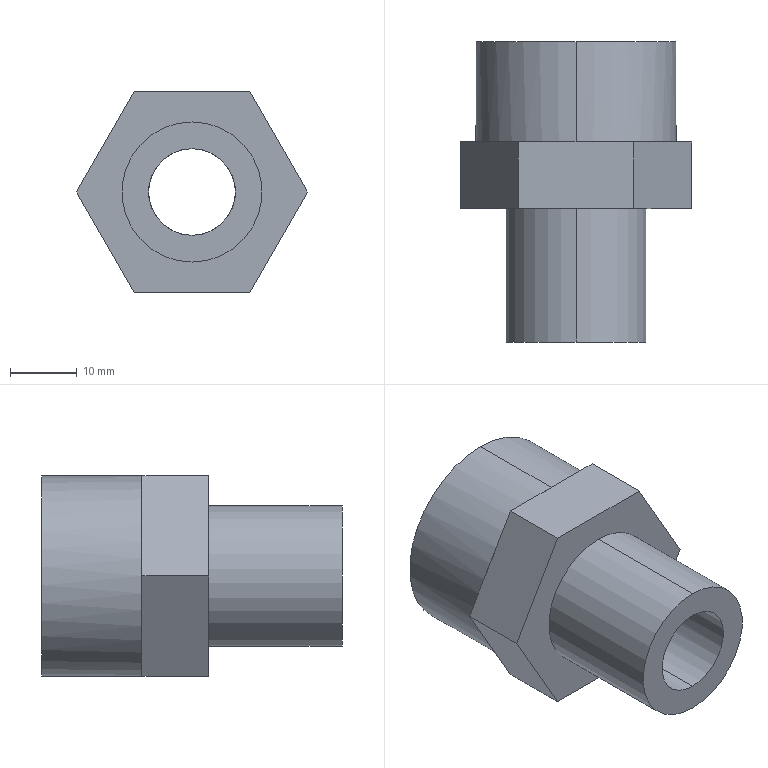Part | 1 solid | 23 faces | box 34.641 x 45 x 30 mm | volume 18087 mm3 | plane 15 | cylinder 6 | cone 2 | commonest cylinder face diameters 13 x2 21 x2 30 x2
STEP:
#1=CARTESIAN_POINT('',(6.5,30.,0.));
#2=VERTEX_POINT('',#1);
#3=CARTESIAN_POINT('',(0.,30.,-6.5));
#4=VERTEX_POINT('',#3);
#5=CARTESIAN_POINT('',(0.,30.,0.));
#6=DIRECTION('',(0.,1.,0.));
#7=DIRECTION('',(-1.,0.,0.));
#8=AXIS2_PLACEMENT_3D('',#5,#6,#7);
#9=CIRCLE('',#8,6.5);
#10=EDGE_CURVE('',#2,#4,#9,.T.);
#11=ORIENTED_EDGE('',*,*,#10,.F.);
#12=CARTESIAN_POINT('',(10.,45.,0.));
#13=VERTEX_POINT('',#12);
#14=CARTESIAN_POINT('',(10.,45.,0.));
#15=DIRECTION('',(0.2272,0.9738,0.));
#16=VECTOR('',#15,1000.);
#17=LINE('',#14,#16);
#18=EDGE_CURVE('',#2,#13,#17,.T.);
#19=ORIENTED_EDGE('',*,*,#18,.T.);
#20=CARTESIAN_POINT('',(-10.,45.,0.));
#21=VERTEX_POINT('',#20);
#22=CARTESIAN_POINT('',(0.,45.,0.));
#23=DIRECTION('',(0.,1.,0.));
#24=DIRECTION('',(-1.,0.,0.));
#25=AXIS2_PLACEMENT_3D('',#22,#23,#24);
#26=CIRCLE('',#25,10.);
#27=EDGE_CURVE('',#13,#21,#26,.T.);
#28=ORIENTED_EDGE('',*,*,#27,.T.);
#29=CARTESIAN_POINT('',(-6.5,30.,0.));
#30=VERTEX_POINT('',#29);
#31=CARTESIAN_POINT('',(-10.,45.,0.));
#32=DIRECTION('',(-0.2272,0.9738,0.));
#33=VECTOR('',#32,1000.);
#34=LINE('',#31,#33);
#35=EDGE_CURVE('',#30,#21,#34,.T.);
#36=ORIENTED_EDGE('',*,*,#35,.F.);
#37=CARTESIAN_POINT('',(0.,30.,0.));
#38=DIRECTION('',(0.,1.,0.));
#39=DIRECTION('',(-1.,0.,0.));
#40=AXIS2_PLACEMENT_3D('',#37,#38,#39);
#41=CIRCLE('',#40,6.5);
#42=EDGE_CURVE('',#4,#30,#41,.T.);
#43=ORIENTED_EDGE('',*,*,#42,.F.);
#44=EDGE_LOOP('',(#11,#19,#28,#36,#43));
#45=FACE_OUTER_BOUND('',#44,.T.);
#46=CARTESIAN_POINT('',(0.,45.,0.));
#47=DIRECTION('',(0.,1.,0.));
#48=DIRECTION('',(-1.,0.,0.));
#49=AXIS2_PLACEMENT_3D('',#46,#47,#48);
#50=CONICAL_SURFACE('',#49,10.,0.2292);
#51=ADVANCED_FACE('',(#45),#50,.F.);
#52=CARTESIAN_POINT('',(0.,0.,-6.5));
#53=VERTEX_POINT('',#52);
#54=CARTESIAN_POINT('',(0.,0.,6.5));
#55=VERTEX_POINT('',#54);
#56=CARTESIAN_POINT('',(0.,0.,0.));
#57=DIRECTION('',(0.,1.,0.));
#58=DIRECTION('',(0.,0.,1.));
#59=AXIS2_PLACEMENT_3D('',#56,#57,#58);
#60=CIRCLE('',#59,6.5);
#61=EDGE_CURVE('',#53,#55,#60,.T.);
#62=ORIENTED_EDGE('',*,*,#61,.F.);
#63=CARTESIAN_POINT('',(0.,0.,-6.5));
#64=DIRECTION('',(0.,1.,0.));
#65=VECTOR('',#64,1000.);
#66=LINE('',#63,#65);
#67=EDGE_CURVE('',#53,#4,#66,.T.);
#68=ORIENTED_EDGE('',*,*,#67,.T.);
#69=ORIENTED_EDGE('',*,*,#42,.T.);
#70=CARTESIAN_POINT('',(0.,30.,6.5));
#71=VERTEX_POINT('',#70);
#72=CARTESIAN_POINT('',(0.,30.,0.));
#73=DIRECTION('',(0.,1.,0.));
#74=DIRECTION('',(-1.,0.,0.));
#75=AXIS2_PLACEMENT_3D('',#72,#73,#74);
#76=CIRCLE('',#75,6.5);
#77=EDGE_CURVE('',#30,#71,#76,.T.);
#78=ORIENTED_EDGE('',*,*,#77,.T.);
#79=CARTESIAN_POINT('',(0.,0.,6.5));
#80=DIRECTION('',(0.,1.,0.));
#81=VECTOR('',#80,1000.);
#82=LINE('',#79,#81);
#83=EDGE_CURVE('',#55,#71,#82,.T.);
#84=ORIENTED_EDGE('',*,*,#83,.F.);
#85=EDGE_LOOP('',(#62,#68,#69,#78,#84));
#86=FACE_OUTER_BOUND('',#85,.T.);
#87=CARTESIAN_POINT('',(0.,0.,0.));
#88=DIRECTION('',(0.,1.,0.));
#89=DIRECTION('',(0.,0.,1.));
#90=AXIS2_PLACEMENT_3D('',#87,#88,#89);
#91=CYLINDRICAL_SURFACE('',#90,6.5);
#92=ADVANCED_FACE('',(#86),#91,.F.);
#93=CARTESIAN_POINT('',(0.,45.,15.));
#94=VERTEX_POINT('',#93);
#95=CARTESIAN_POINT('',(0.,45.,-15.));
#96=VERTEX_POINT('',#95);
#97=CARTESIAN_POINT('',(0.,45.,0.));
#98=DIRECTION('',(0.,1.,0.));
#99=DIRECTION('',(0.,0.,1.));
#100=AXIS2_PLACEMENT_3D('',#97,#98,#99);
#101=CIRCLE('',#100,15.);
#102=EDGE_CURVE('',#94,#96,#101,.T.);
#103=ORIENTED_EDGE('',*,*,#102,.F.);
#104=CARTESIAN_POINT('',(0.,30.,15.));
#105=VERTEX_POINT('',#104);
#106=CARTESIAN_POINT('',(0.,87.426,15.));
#107=DIRECTION('',(0.,-1.,0.));
#108=VECTOR('',#107,1000.);
#109=LINE('',#106,#108);
#110=EDGE_CURVE('',#94,#105,#109,.T.);
#111=ORIENTED_EDGE('',*,*,#110,.T.);
#112=CARTESIAN_POINT('',(12.99,30.,7.5));
#113=VERTEX_POINT('',#112);
#114=CARTESIAN_POINT('',(0.,30.,0.));
#115=DIRECTION('',(0.,1.,0.));
#116=DIRECTION('',(0.,0.,1.));
#117=AXIS2_PLACEMENT_3D('',#114,#115,#116);
#118=CIRCLE('',#117,15.);
#119=EDGE_CURVE('',#105,#113,#118,.T.);
#120=ORIENTED_EDGE('',*,*,#119,.T.);
#121=CARTESIAN_POINT('',(12.99,30.,-7.5));
#122=VERTEX_POINT('',#121);
#123=CARTESIAN_POINT('',(0.,30.,0.));
#124=DIRECTION('',(0.,1.,0.));
#125=DIRECTION('',(0.,0.,1.));
#126=AXIS2_PLACEMENT_3D('',#123,#124,#125);
#127=CIRCLE('',#126,15.);
#128=EDGE_CURVE('',#113,#122,#127,.T.);
#129=ORIENTED_EDGE('',*,*,#128,.T.);
#130=CARTESIAN_POINT('',(0.,30.,-15.));
#131=VERTEX_POINT('',#130);
#132=CARTESIAN_POINT('',(0.,30.,0.));
#133=DIRECTION('',(0.,1.,0.));
#134=DIRECTION('',(0.,0.,1.));
#135=AXIS2_PLACEMENT_3D('',#132,#133,#134);
#136=CIRCLE('',#135,15.);
#137=EDGE_CURVE('',#122,#131,#136,.T.);
#138=ORIENTED_EDGE('',*,*,#137,.T.);
#139=CARTESIAN_POINT('',(0.,87.426,-15.));
#140=DIRECTION('',(0.,-1.,0.));
#141=VECTOR('',#140,1000.);
#142=LINE('',#139,#141);
#143=EDGE_CURVE('',#96,#131,#142,.T.);
#144=ORIENTED_EDGE('',*,*,#143,.F.);
#145=EDGE_LOOP('',(#103,#111,#120,#129,#138,#144));
#146=FACE_OUTER_BOUND('',#145,.T.);
#147=CARTESIAN_POINT('',(0.,87.426,0.));
#148=DIRECTION('',(0.,-1.,0.));
#149=DIRECTION('',(0.,0.,-1.));
#150=AXIS2_PLACEMENT_3D('',#147,#148,#149);
#151=CYLINDRICAL_SURFACE('',#150,15.);
#152=ADVANCED_FACE('',(#146),#151,.T.);
#153=CARTESIAN_POINT('',(0.,20.,10.5));
#154=VERTEX_POINT('',#153);
#155=CARTESIAN_POINT('',(0.,20.,-10.5));
#156=VERTEX_POINT('',#155);
#157=CARTESIAN_POINT('',(0.,20.,0.));
#158=DIRECTION('',(0.,1.,0.));
#159=DIRECTION('',(0.,0.,1.));
#160=AXIS2_PLACEMENT_3D('',#157,#158,#159);
#161=CIRCLE('',#160,10.5);
#162=EDGE_CURVE('',#154,#156,#161,.T.);
#163=ORIENTED_EDGE('',*,*,#162,.F.);
#164=CARTESIAN_POINT('',(0.,0.,10.5));
#165=VERTEX_POINT('',#164);
#166=CARTESIAN_POINT('',(0.,45.,10.5));
#167=DIRECTION('',(0.,-1.,0.));
#168=VECTOR('',#167,1000.);
#169=LINE('',#166,#168);
#170=EDGE_CURVE('',#154,#165,#169,.T.);
#171=ORIENTED_EDGE('',*,*,#170,.T.);
#172=CARTESIAN_POINT('',(0.,0.,-10.5));
#173=VERTEX_POINT('',#172);
#174=CARTESIAN_POINT('',(0.,0.,0.));
#175=DIRECTION('',(0.,1.,0.));
#176=DIRECTION('',(0.,0.,1.));
#177=AXIS2_PLACEMENT_3D('',#174,#175,#176);
#178=CIRCLE('',#177,10.5);
#179=EDGE_CURVE('',#165,#173,#178,.T.);
#180=ORIENTED_EDGE('',*,*,#179,.T.);
#181=CARTESIAN_POINT('',(0.,45.,-10.5));
#182=DIRECTION('',(0.,-1.,0.));
#183=VECTOR('',#182,1000.);
#184=LINE('',#181,#183);
#185=EDGE_CURVE('',#156,#173,#184,.T.);
#186=ORIENTED_EDGE('',*,*,#185,.F.);
#187=EDGE_LOOP('',(#163,#171,#180,#186));
#188=FACE_OUTER_BOUND('',#187,.T.);
#189=CARTESIAN_POINT('',(0.,45.,0.));
#190=DIRECTION('',(0.,-1.,0.));
#191=DIRECTION('',(0.,0.,-1.));
#192=AXIS2_PLACEMENT_3D('',#189,#190,#191);
#193=CYLINDRICAL_SURFACE('',#192,10.5);
#194=ADVANCED_FACE('',(#188),#193,.T.);
#195=ORIENTED_EDGE('',*,*,#170,.F.);
#196=CARTESIAN_POINT('',(0.,20.,0.));
#197=DIRECTION('',(0.,1.,0.));
#198=DIRECTION('',(0.,0.,1.));
#199=AXIS2_PLACEMENT_3D('',#196,#197,#198);
#200=CIRCLE('',#199,10.5);
#201=EDGE_CURVE('',#156,#154,#200,.T.);
#202=ORIENTED_EDGE('',*,*,#201,.F.);
#203=ORIENTED_EDGE('',*,*,#185,.T.);
#204=CARTESIAN_POINT('',(0.,0.,0.));
#205=DIRECTION('',(0.,1.,0.));
#206=DIRECTION('',(0.,0.,1.));
#207=AXIS2_PLACEMENT_3D('',#204,#205,#206);
#208=CIRCLE('',#207,10.5);
#209=EDGE_CURVE('',#173,#165,#208,.T.);
#210=ORIENTED_EDGE('',*,*,#209,.T.);
#211=EDGE_LOOP('',(#195,#202,#203,#210));
#212=FACE_OUTER_BOUND('',#211,.T.);
#213=CARTESIAN_POINT('',(0.,45.,0.));
#214=DIRECTION('',(0.,-1.,0.));
#215=DIRECTION('',(0.,0.,-1.));
#216=AXIS2_PLACEMENT_3D('',#213,#214,#215);
#217=CYLINDRICAL_SURFACE('',#216,10.5);
#218=ADVANCED_FACE('',(#212),#217,.T.);
#219=CARTESIAN_POINT('',(0.,0.,0.));
#220=DIRECTION('',(0.,1.,0.));
#221=DIRECTION('',(0.,0.,1.));
#222=AXIS2_PLACEMENT_3D('',#219,#220,#221);
#223=CIRCLE('',#222,6.5);
#224=EDGE_CURVE('',#55,#53,#223,.T.);
#225=ORIENTED_EDGE('',*,*,#224,.T.);
#226=ORIENTED_EDGE('',*,*,#61,.T.);
#227=EDGE_LOOP('',(#225,#226));
#228=FACE_BOUND('',#227,.T.);
#229=ORIENTED_EDGE('',*,*,#209,.F.);
#230=ORIENTED_EDGE('',*,*,#179,.F.);
#231=EDGE_LOOP('',(#229,#230));
#232=FACE_OUTER_BOUND('',#231,.T.);
#233=CARTESIAN_POINT('',(0.,0.,0.));
#234=DIRECTION('',(0.,1.,0.));
#235=DIRECTION('',(0.,0.,1.));
#236=AXIS2_PLACEMENT_3D('',#233,#234,#235);
#237=PLANE('',#236);
#238=ADVANCED_FACE('',(#228,#232),#237,.F.);
#239=ORIENTED_EDGE('',*,*,#201,.T.);
#240=ORIENTED_EDGE('',*,*,#162,.T.);
#241=EDGE_LOOP('',(#239,#240));
#242=FACE_BOUND('',#241,.T.);
#243=CARTESIAN_POINT('',(8.66,20.,15.));
#244=VERTEX_POINT('',#243);
#245=CARTESIAN_POINT('',(17.321,20.,0.));
#246=VERTEX_POINT('',#245);
#247=CARTESIAN_POINT('',(8.66,20.,15.));
#248=DIRECTION('',(0.5,0.,-0.866));
#249=VECTOR('',#248,1000.);
#250=LINE('',#247,#249);
#251=EDGE_CURVE('',#244,#246,#250,.T.);
#252=ORIENTED_EDGE('',*,*,#251,.F.);
#253=CARTESIAN_POINT('',(-8.66,20.,15.));
#254=VERTEX_POINT('',#253);
#255=CARTESIAN_POINT('',(-8.66,20.,15.));
#256=DIRECTION('',(1.,0.,0.));
#257=VECTOR('',#256,1000.);
#258=LINE('',#255,#257);
#259=EDGE_CURVE('',#254,#244,#258,.T.);
#260=ORIENTED_EDGE('',*,*,#259,.F.);
#261=CARTESIAN_POINT('',(-17.321,20.,0.));
#262=VERTEX_POINT('',#261);
#263=CARTESIAN_POINT('',(-17.321,20.,0.));
#264=DIRECTION('',(0.5,0.,0.866));
#265=VECTOR('',#264,1000.);
#266=LINE('',#263,#265);
#267=EDGE_CURVE('',#262,#254,#266,.T.);
#268=ORIENTED_EDGE('',*,*,#267,.F.);
#269=CARTESIAN_POINT('',(-8.66,20.,-15.));
#270=VERTEX_POINT('',#269);
#271=CARTESIAN_POINT('',(-8.66,20.,-15.));
#272=DIRECTION('',(-0.5,0.,0.866));
#273=VECTOR('',#272,1000.);
#274=LINE('',#271,#273);
#275=EDGE_CURVE('',#270,#262,#274,.T.);
#276=ORIENTED_EDGE('',*,*,#275,.F.);
#277=CARTESIAN_POINT('',(8.66,20.,-15.));
#278=VERTEX_POINT('',#277);
#279=CARTESIAN_POINT('',(8.66,20.,-15.));
#280=DIRECTION('',(-1.,0.,0.));
#281=VECTOR('',#280,1000.);
#282=LINE('',#279,#281);
#283=EDGE_CURVE('',#278,#270,#282,.T.);
#284=ORIENTED_EDGE('',*,*,#283,.F.);
#285=CARTESIAN_POINT('',(17.321,20.,0.));
#286=DIRECTION('',(-0.5,0.,-0.866));
#287=VECTOR('',#286,1000.);
#288=LINE('',#285,#287);
#289=EDGE_CURVE('',#246,#278,#288,.T.);
#290=ORIENTED_EDGE('',*,*,#289,.F.);
#291=EDGE_LOOP('',(#252,#260,#268,#276,#284,#290));
#292=FACE_OUTER_BOUND('',#291,.T.);
#293=CARTESIAN_POINT('',(0.,20.,0.));
#294=DIRECTION('',(0.,1.,0.));
#295=DIRECTION('',(0.,0.,1.));
#296=AXIS2_PLACEMENT_3D('',#293,#294,#295);
#297=PLANE('',#296);
#298=ADVANCED_FACE('',(#242,#292),#297,.F.);
#299=ORIENTED_EDGE('',*,*,#119,.F.);
#300=CARTESIAN_POINT('',(8.66,30.,15.));
#301=VERTEX_POINT('',#300);
#302=CARTESIAN_POINT('',(-8.66,30.,15.));
#303=DIRECTION('',(1.,0.,0.));
#304=VECTOR('',#303,1000.);
#305=LINE('',#302,#304);
#306=EDGE_CURVE('',#105,#301,#305,.T.);
#307=ORIENTED_EDGE('',*,*,#306,.T.);
#308=CARTESIAN_POINT('',(8.66,30.,15.));
#309=DIRECTION('',(0.5,0.,-0.866));
#310=VECTOR('',#309,1000.);
#311=LINE('',#308,#310);
#312=EDGE_CURVE('',#301,#113,#311,.T.);
#313=ORIENTED_EDGE('',*,*,#312,.T.);
#314=EDGE_LOOP('',(#299,#307,#313));
#315=FACE_OUTER_BOUND('',#314,.T.);
#316=CARTESIAN_POINT('',(0.,30.,0.));
#317=DIRECTION('',(0.,1.,0.));
#318=DIRECTION('',(0.,0.,1.));
#319=AXIS2_PLACEMENT_3D('',#316,#317,#318);
#320=PLANE('',#319);
#321=ADVANCED_FACE('',(#315),#320,.T.);
#322=ORIENTED_EDGE('',*,*,#128,.F.);
#323=CARTESIAN_POINT('',(17.321,30.,0.));
#324=VERTEX_POINT('',#323);
#325=CARTESIAN_POINT('',(8.66,30.,15.));
#326=DIRECTION('',(0.5,0.,-0.866));
#327=VECTOR('',#326,1000.);
#328=LINE('',#325,#327);
#329=EDGE_CURVE('',#113,#324,#328,.T.);
#330=ORIENTED_EDGE('',*,*,#329,.T.);
#331=CARTESIAN_POINT('',(17.321,30.,0.));
#332=DIRECTION('',(-0.5,0.,-0.866));
#333=VECTOR('',#332,1000.);
#334=LINE('',#331,#333);
#335=EDGE_CURVE('',#324,#122,#334,.T.);
#336=ORIENTED_EDGE('',*,*,#335,.T.);
#337=EDGE_LOOP('',(#322,#330,#336));
#338=FACE_OUTER_BOUND('',#337,.T.);
#339=CARTESIAN_POINT('',(0.,30.,0.));
#340=DIRECTION('',(0.,1.,0.));
#341=DIRECTION('',(0.,0.,1.));
#342=AXIS2_PLACEMENT_3D('',#339,#340,#341);
#343=PLANE('',#342);
#344=ADVANCED_FACE('',(#338),#343,.T.);
#345=ORIENTED_EDGE('',*,*,#137,.F.);
#346=CARTESIAN_POINT('',(8.66,30.,-15.));
#347=VERTEX_POINT('',#346);
#348=CARTESIAN_POINT('',(17.321,30.,0.));
#349=DIRECTION('',(-0.5,0.,-0.866));
#350=VECTOR('',#349,1000.);
#351=LINE('',#348,#350);
#352=EDGE_CURVE('',#122,#347,#351,.T.);
#353=ORIENTED_EDGE('',*,*,#352,.T.);
#354=CARTESIAN_POINT('',(8.66,30.,-15.));
#355=DIRECTION('',(-1.,0.,0.));
#356=VECTOR('',#355,1000.);
#357=LINE('',#354,#356);
#358=EDGE_CURVE('',#347,#131,#357,.T.);
#359=ORIENTED_EDGE('',*,*,#358,.T.);
#360=EDGE_LOOP('',(#345,#353,#359));
#361=FACE_OUTER_BOUND('',#360,.T.);
#362=CARTESIAN_POINT('',(0.,30.,0.));
#363=DIRECTION('',(0.,1.,0.));
#364=DIRECTION('',(0.,0.,1.));
#365=AXIS2_PLACEMENT_3D('',#362,#363,#364);
#366=PLANE('',#365);
#367=ADVANCED_FACE('',(#361),#366,.T.);
#368=CARTESIAN_POINT('',(-12.99,30.,-7.5));
#369=VERTEX_POINT('',#368);
#370=CARTESIAN_POINT('',(0.,30.,0.));
#371=DIRECTION('',(0.,1.,0.));
#372=DIRECTION('',(0.,0.,1.));
#373=AXIS2_PLACEMENT_3D('',#370,#371,#372);
#374=CIRCLE('',#373,15.);
#375=EDGE_CURVE('',#131,#369,#374,.T.);
#376=ORIENTED_EDGE('',*,*,#375,.F.);
#377=CARTESIAN_POINT('',(-8.66,30.,-15.));
#378=VERTEX_POINT('',#377);
#379=CARTESIAN_POINT('',(8.66,30.,-15.));
#380=DIRECTION('',(-1.,0.,0.));
#381=VECTOR('',#380,1000.);
#382=LINE('',#379,#381);
#383=EDGE_CURVE('',#131,#378,#382,.T.);
#384=ORIENTED_EDGE('',*,*,#383,.T.);
#385=CARTESIAN_POINT('',(-8.66,30.,-15.));
#386=DIRECTION('',(-0.5,0.,0.866));
#387=VECTOR('',#386,1000.);
#388=LINE('',#385,#387);
#389=EDGE_CURVE('',#378,#369,#388,.T.);
#390=ORIENTED_EDGE('',*,*,#389,.T.);
#391=EDGE_LOOP('',(#376,#384,#390));
#392=FACE_OUTER_BOUND('',#391,.T.);
#393=CARTESIAN_POINT('',(0.,30.,0.));
#394=DIRECTION('',(0.,1.,0.));
#395=DIRECTION('',(0.,0.,1.));
#396=AXIS2_PLACEMENT_3D('',#393,#394,#395);
#397=PLANE('',#396);
#398=ADVANCED_FACE('',(#392),#397,.T.);
#399=CARTESIAN_POINT('',(-12.99,30.,7.5));
#400=VERTEX_POINT('',#399);
#401=CARTESIAN_POINT('',(0.,30.,0.));
#402=DIRECTION('',(0.,1.,0.));
#403=DIRECTION('',(0.,0.,1.));
#404=AXIS2_PLACEMENT_3D('',#401,#402,#403);
#405=CIRCLE('',#404,15.);
#406=EDGE_CURVE('',#369,#400,#405,.T.);
#407=ORIENTED_EDGE('',*,*,#406,.F.);
#408=CARTESIAN_POINT('',(-17.321,30.,0.));
#409=VERTEX_POINT('',#408);
#410=CARTESIAN_POINT('',(-8.66,30.,-15.));
#411=DIRECTION('',(-0.5,0.,0.866));
#412=VECTOR('',#411,1000.);
#413=LINE('',#410,#412);
#414=EDGE_CURVE('',#369,#409,#413,.T.);
#415=ORIENTED_EDGE('',*,*,#414,.T.);
#416=CARTESIAN_POINT('',(-17.321,30.,0.));
#417=DIRECTION('',(0.5,0.,0.866));
#418=VECTOR('',#417,1000.);
#419=LINE('',#416,#418);
#420=EDGE_CURVE('',#409,#400,#419,.T.);
#421=ORIENTED_EDGE('',*,*,#420,.T.);
#422=EDGE_LOOP('',(#407,#415,#421));
#423=FACE_OUTER_BOUND('',#422,.T.);
#424=CARTESIAN_POINT('',(0.,30.,0.));
#425=DIRECTION('',(0.,1.,0.));
#426=DIRECTION('',(0.,0.,1.));
#427=AXIS2_PLACEMENT_3D('',#424,#425,#426);
#428=PLANE('',#427);
#429=ADVANCED_FACE('',(#423),#428,.T.);
#430=ORIENTED_EDGE('',*,*,#352,.F.);
#431=ORIENTED_EDGE('',*,*,#335,.F.);
#432=CARTESIAN_POINT('',(17.321,30.,0.));
#433=DIRECTION('',(0.,-1.,0.));
#434=VECTOR('',#433,1000.);
#435=LINE('',#432,#434);
#436=EDGE_CURVE('',#324,#246,#435,.T.);
#437=ORIENTED_EDGE('',*,*,#436,.T.);
#438=ORIENTED_EDGE('',*,*,#289,.T.);
#439=CARTESIAN_POINT('',(8.66,30.,-15.));
#440=DIRECTION('',(0.,-1.,0.));
#441=VECTOR('',#440,1000.);
#442=LINE('',#439,#441);
#443=EDGE_CURVE('',#347,#278,#442,.T.);
#444=ORIENTED_EDGE('',*,*,#443,.F.);
#445=EDGE_LOOP('',(#430,#431,#437,#438,#444));
#446=FACE_OUTER_BOUND('',#445,.T.);
#447=CARTESIAN_POINT('',(17.321,30.,0.));
#448=DIRECTION('',(-0.866,0.,0.5));
#449=DIRECTION('',(0.5,0.,0.866));
#450=AXIS2_PLACEMENT_3D('',#447,#448,#449);
#451=PLANE('',#450);
#452=ADVANCED_FACE('',(#446),#451,.F.);
#453=ORIENTED_EDGE('',*,*,#383,.F.);
#454=ORIENTED_EDGE('',*,*,#358,.F.);
#455=ORIENTED_EDGE('',*,*,#443,.T.);
#456=ORIENTED_EDGE('',*,*,#283,.T.);
#457=CARTESIAN_POINT('',(-8.66,30.,-15.));
#458=DIRECTION('',(0.,-1.,0.));
#459=VECTOR('',#458,1000.);
#460=LINE('',#457,#459);
#461=EDGE_CURVE('',#378,#270,#460,.T.);
#462=ORIENTED_EDGE('',*,*,#461,.F.);
#463=EDGE_LOOP('',(#453,#454,#455,#456,#462));
#464=FACE_OUTER_BOUND('',#463,.T.);
#465=CARTESIAN_POINT('',(8.66,30.,-15.));
#466=DIRECTION('',(0.,0.,1.));
#467=DIRECTION('',(1.,0.,0.));
#468=AXIS2_PLACEMENT_3D('',#465,#466,#467);
#469=PLANE('',#468);
#470=ADVANCED_FACE('',(#464),#469,.F.);
#471=ORIENTED_EDGE('',*,*,#414,.F.);
#472=ORIENTED_EDGE('',*,*,#389,.F.);
#473=ORIENTED_EDGE('',*,*,#461,.T.);
#474=ORIENTED_EDGE('',*,*,#275,.T.);
#475=CARTESIAN_POINT('',(-17.321,30.,0.));
#476=DIRECTION('',(0.,-1.,0.));
#477=VECTOR('',#476,1000.);
#478=LINE('',#475,#477);
#479=EDGE_CURVE('',#409,#262,#478,.T.);
#480=ORIENTED_EDGE('',*,*,#479,.F.);
#481=EDGE_LOOP('',(#471,#472,#473,#474,#480));
#482=FACE_OUTER_BOUND('',#481,.T.);
#483=CARTESIAN_POINT('',(-8.66,30.,-15.));
#484=DIRECTION('',(0.866,0.,0.5));
#485=DIRECTION('',(0.5,0.,-0.866));
#486=AXIS2_PLACEMENT_3D('',#483,#484,#485);
#487=PLANE('',#486);
#488=ADVANCED_FACE('',(#482),#487,.F.);
#489=CARTESIAN_POINT('',(-8.66,30.,15.));
#490=VERTEX_POINT('',#489);
#491=CARTESIAN_POINT('',(-17.321,30.,0.));
#492=DIRECTION('',(0.5,0.,0.866));
#493=VECTOR('',#492,1000.);
#494=LINE('',#491,#493);
#495=EDGE_CURVE('',#400,#490,#494,.T.);
#496=ORIENTED_EDGE('',*,*,#495,.F.);
#497=ORIENTED_EDGE('',*,*,#420,.F.);
#498=ORIENTED_EDGE('',*,*,#479,.T.);
#499=ORIENTED_EDGE('',*,*,#267,.T.);
#500=CARTESIAN_POINT('',(-8.66,30.,15.));
#501=DIRECTION('',(0.,-1.,0.));
#502=VECTOR('',#501,1000.);
#503=LINE('',#500,#502);
#504=EDGE_CURVE('',#490,#254,#503,.T.);
#505=ORIENTED_EDGE('',*,*,#504,.F.);
#506=EDGE_LOOP('',(#496,#497,#498,#499,#505));
#507=FACE_OUTER_BOUND('',#506,.T.);
#508=CARTESIAN_POINT('',(-17.321,30.,0.));
#509=DIRECTION('',(0.866,0.,-0.5));
#510=DIRECTION('',(-0.5,0.,-0.866));
#511=AXIS2_PLACEMENT_3D('',#508,#509,#510);
#512=PLANE('',#511);
#513=ADVANCED_FACE('',(#507),#512,.F.);
#514=ORIENTED_EDGE('',*,*,#306,.F.);
#515=CARTESIAN_POINT('',(-8.66,30.,15.));
#516=DIRECTION('',(1.,0.,0.));
#517=VECTOR('',#516,1000.);
#518=LINE('',#515,#517);
#519=EDGE_CURVE('',#490,#105,#518,.T.);
#520=ORIENTED_EDGE('',*,*,#519,.F.);
#521=ORIENTED_EDGE('',*,*,#504,.T.);
#522=ORIENTED_EDGE('',*,*,#259,.T.);
#523=CARTESIAN_POINT('',(8.66,30.,15.));
#524=DIRECTION('',(0.,-1.,0.));
#525=VECTOR('',#524,1000.);
#526=LINE('',#523,#525);
#527=EDGE_CURVE('',#301,#244,#526,.T.);
#528=ORIENTED_EDGE('',*,*,#527,.F.);
#529=EDGE_LOOP('',(#514,#520,#521,#522,#528));
#530=FACE_OUTER_BOUND('',#529,.T.);
#531=CARTESIAN_POINT('',(-8.66,30.,15.));
#532=DIRECTION('',(0.,0.,-1.));
#533=DIRECTION('',(-1.,0.,0.));
#534=AXIS2_PLACEMENT_3D('',#531,#532,#533);
#535=PLANE('',#534);
#536=ADVANCED_FACE('',(#530),#535,.F.);
#537=ORIENTED_EDGE('',*,*,#329,.F.);
#538=ORIENTED_EDGE('',*,*,#312,.F.);
#539=ORIENTED_EDGE('',*,*,#527,.T.);
#540=ORIENTED_EDGE('',*,*,#251,.T.);
#541=ORIENTED_EDGE('',*,*,#436,.F.);
#542=EDGE_LOOP('',(#537,#538,#539,#540,#541));
#543=FACE_OUTER_BOUND('',#542,.T.);
#544=CARTESIAN_POINT('',(8.66,30.,15.));
#545=DIRECTION('',(-0.866,0.,-0.5));
#546=DIRECTION('',(-0.5,0.,0.866));
#547=AXIS2_PLACEMENT_3D('',#544,#545,#546);
#548=PLANE('',#547);
#549=ADVANCED_FACE('',(#543),#548,.F.);
#550=CARTESIAN_POINT('',(0.,30.,0.));
#551=DIRECTION('',(0.,1.,0.));
#552=DIRECTION('',(0.,0.,1.));
#553=AXIS2_PLACEMENT_3D('',#550,#551,#552);
#554=CIRCLE('',#553,15.);
#555=EDGE_CURVE('',#400,#105,#554,.T.);
#556=ORIENTED_EDGE('',*,*,#555,.F.);
#557=ORIENTED_EDGE('',*,*,#495,.T.);
#558=ORIENTED_EDGE('',*,*,#519,.T.);
#559=EDGE_LOOP('',(#556,#557,#558));
#560=FACE_OUTER_BOUND('',#559,.T.);
#561=CARTESIAN_POINT('',(0.,30.,0.));
#562=DIRECTION('',(0.,1.,0.));
#563=DIRECTION('',(0.,0.,1.));
#564=AXIS2_PLACEMENT_3D('',#561,#562,#563);
#565=PLANE('',#564);
#566=ADVANCED_FACE('',(#560),#565,.T.);
#567=CARTESIAN_POINT('',(0.,45.,0.));
#568=DIRECTION('',(0.,1.,0.));
#569=DIRECTION('',(-1.,0.,0.));
#570=AXIS2_PLACEMENT_3D('',#567,#568,#569);
#571=CIRCLE('',#570,10.);
#572=EDGE_CURVE('',#21,#13,#571,.T.);
#573=ORIENTED_EDGE('',*,*,#572,.F.);
#574=ORIENTED_EDGE('',*,*,#27,.F.);
#575=EDGE_LOOP('',(#573,#574));
#576=FACE_BOUND('',#575,.T.);
#577=CARTESIAN_POINT('',(0.,45.,0.));
#578=DIRECTION('',(0.,1.,0.));
#579=DIRECTION('',(0.,0.,1.));
#580=AXIS2_PLACEMENT_3D('',#577,#578,#579);
#581=CIRCLE('',#580,15.);
#582=EDGE_CURVE('',#96,#94,#581,.T.);
#583=ORIENTED_EDGE('',*,*,#582,.T.);
#584=ORIENTED_EDGE('',*,*,#102,.T.);
#585=EDGE_LOOP('',(#583,#584));
#586=FACE_OUTER_BOUND('',#585,.T.);
#587=CARTESIAN_POINT('',(0.,45.,0.));
#588=DIRECTION('',(0.,1.,0.));
#589=DIRECTION('',(0.,0.,1.));
#590=AXIS2_PLACEMENT_3D('',#587,#588,#589);
#591=PLANE('',#590);
#592=ADVANCED_FACE('',(#576,#586),#591,.T.);
#593=ORIENTED_EDGE('',*,*,#110,.F.);
#594=ORIENTED_EDGE('',*,*,#582,.F.);
#595=ORIENTED_EDGE('',*,*,#143,.T.);
#596=ORIENTED_EDGE('',*,*,#375,.T.);
#597=ORIENTED_EDGE('',*,*,#406,.T.);
#598=ORIENTED_EDGE('',*,*,#555,.T.);
#599=EDGE_LOOP('',(#593,#594,#595,#596,#597,#598));
#600=FACE_OUTER_BOUND('',#599,.T.);
#601=CARTESIAN_POINT('',(0.,87.426,0.));
#602=DIRECTION('',(0.,-1.,0.));
#603=DIRECTION('',(0.,0.,-1.));
#604=AXIS2_PLACEMENT_3D('',#601,#602,#603);
#605=CYLINDRICAL_SURFACE('',#604,15.);
#606=ADVANCED_FACE('',(#600),#605,.T.);
#607=ORIENTED_EDGE('',*,*,#67,.F.);
#608=ORIENTED_EDGE('',*,*,#224,.F.);
#609=ORIENTED_EDGE('',*,*,#83,.T.);
#610=CARTESIAN_POINT('',(0.,30.,0.));
#611=DIRECTION('',(0.,1.,0.));
#612=DIRECTION('',(-1.,0.,0.));
#613=AXIS2_PLACEMENT_3D('',#610,#611,#612);
#614=CIRCLE('',#613,6.5);
#615=EDGE_CURVE('',#71,#2,#614,.T.);
#616=ORIENTED_EDGE('',*,*,#615,.T.);
#617=ORIENTED_EDGE('',*,*,#10,.T.);
#618=EDGE_LOOP('',(#607,#608,#609,#616,#617));
#619=FACE_OUTER_BOUND('',#618,.T.);
#620=CARTESIAN_POINT('',(0.,0.,0.));
#621=DIRECTION('',(0.,1.,0.));
#622=DIRECTION('',(0.,0.,1.));
#623=AXIS2_PLACEMENT_3D('',#620,#621,#622);
#624=CYLINDRICAL_SURFACE('',#623,6.5);
#625=ADVANCED_FACE('',(#619),#624,.F.);
#626=ORIENTED_EDGE('',*,*,#18,.F.);
#627=ORIENTED_EDGE('',*,*,#615,.F.);
#628=ORIENTED_EDGE('',*,*,#77,.F.);
#629=ORIENTED_EDGE('',*,*,#35,.T.);
#630=ORIENTED_EDGE('',*,*,#572,.T.);
#631=EDGE_LOOP('',(#626,#627,#628,#629,#630));
#632=FACE_OUTER_BOUND('',#631,.T.);
#633=CARTESIAN_POINT('',(0.,45.,0.));
#634=DIRECTION('',(0.,1.,0.));
#635=DIRECTION('',(-1.,0.,0.));
#636=AXIS2_PLACEMENT_3D('',#633,#634,#635);
#637=CONICAL_SURFACE('',#636,10.,0.2292);
#638=ADVANCED_FACE('',(#632),#637,.F.);
#639=CLOSED_SHELL('',(#51,#92,#152,#194,#218,#238,#298,#321,#344,#367,#398,#429,#452,#470,#488,#513,#536,#549,#566,#592,#606,#625,#638));
#640=MANIFOLD_SOLID_BREP('',#639);
#641=CARTESIAN_POINT('',(0.,0.,0.));
#642=DIRECTION('',(0.,0.,1.));
#643=DIRECTION('',(1.,0.,0.));
#644=AXIS2_PLACEMENT_3D('',#641,#642,#643);
#645=(LENGTH_UNIT()NAMED_UNIT(*)SI_UNIT(.MILLI.,.METRE.));
#646=UNCERTAINTY_MEASURE_WITH_UNIT(LENGTH_MEASURE(0.00001),#645,'','');
#647=(NAMED_UNIT(*)PLANE_ANGLE_UNIT()SI_UNIT($,.RADIAN.));
#648=(NAMED_UNIT(*)SI_UNIT($,.STERADIAN.)SOLID_ANGLE_UNIT());
#649=(GEOMETRIC_REPRESENTATION_CONTEXT(3)GLOBAL_UNCERTAINTY_ASSIGNED_CONTEXT((#646))GLOBAL_UNIT_ASSIGNED_CONTEXT((#645,#647,#648))REPRESENTATION_CONTEXT('',''));
#650=ADVANCED_BREP_SHAPE_REPRESENTATION('',(#640,#644),#649);